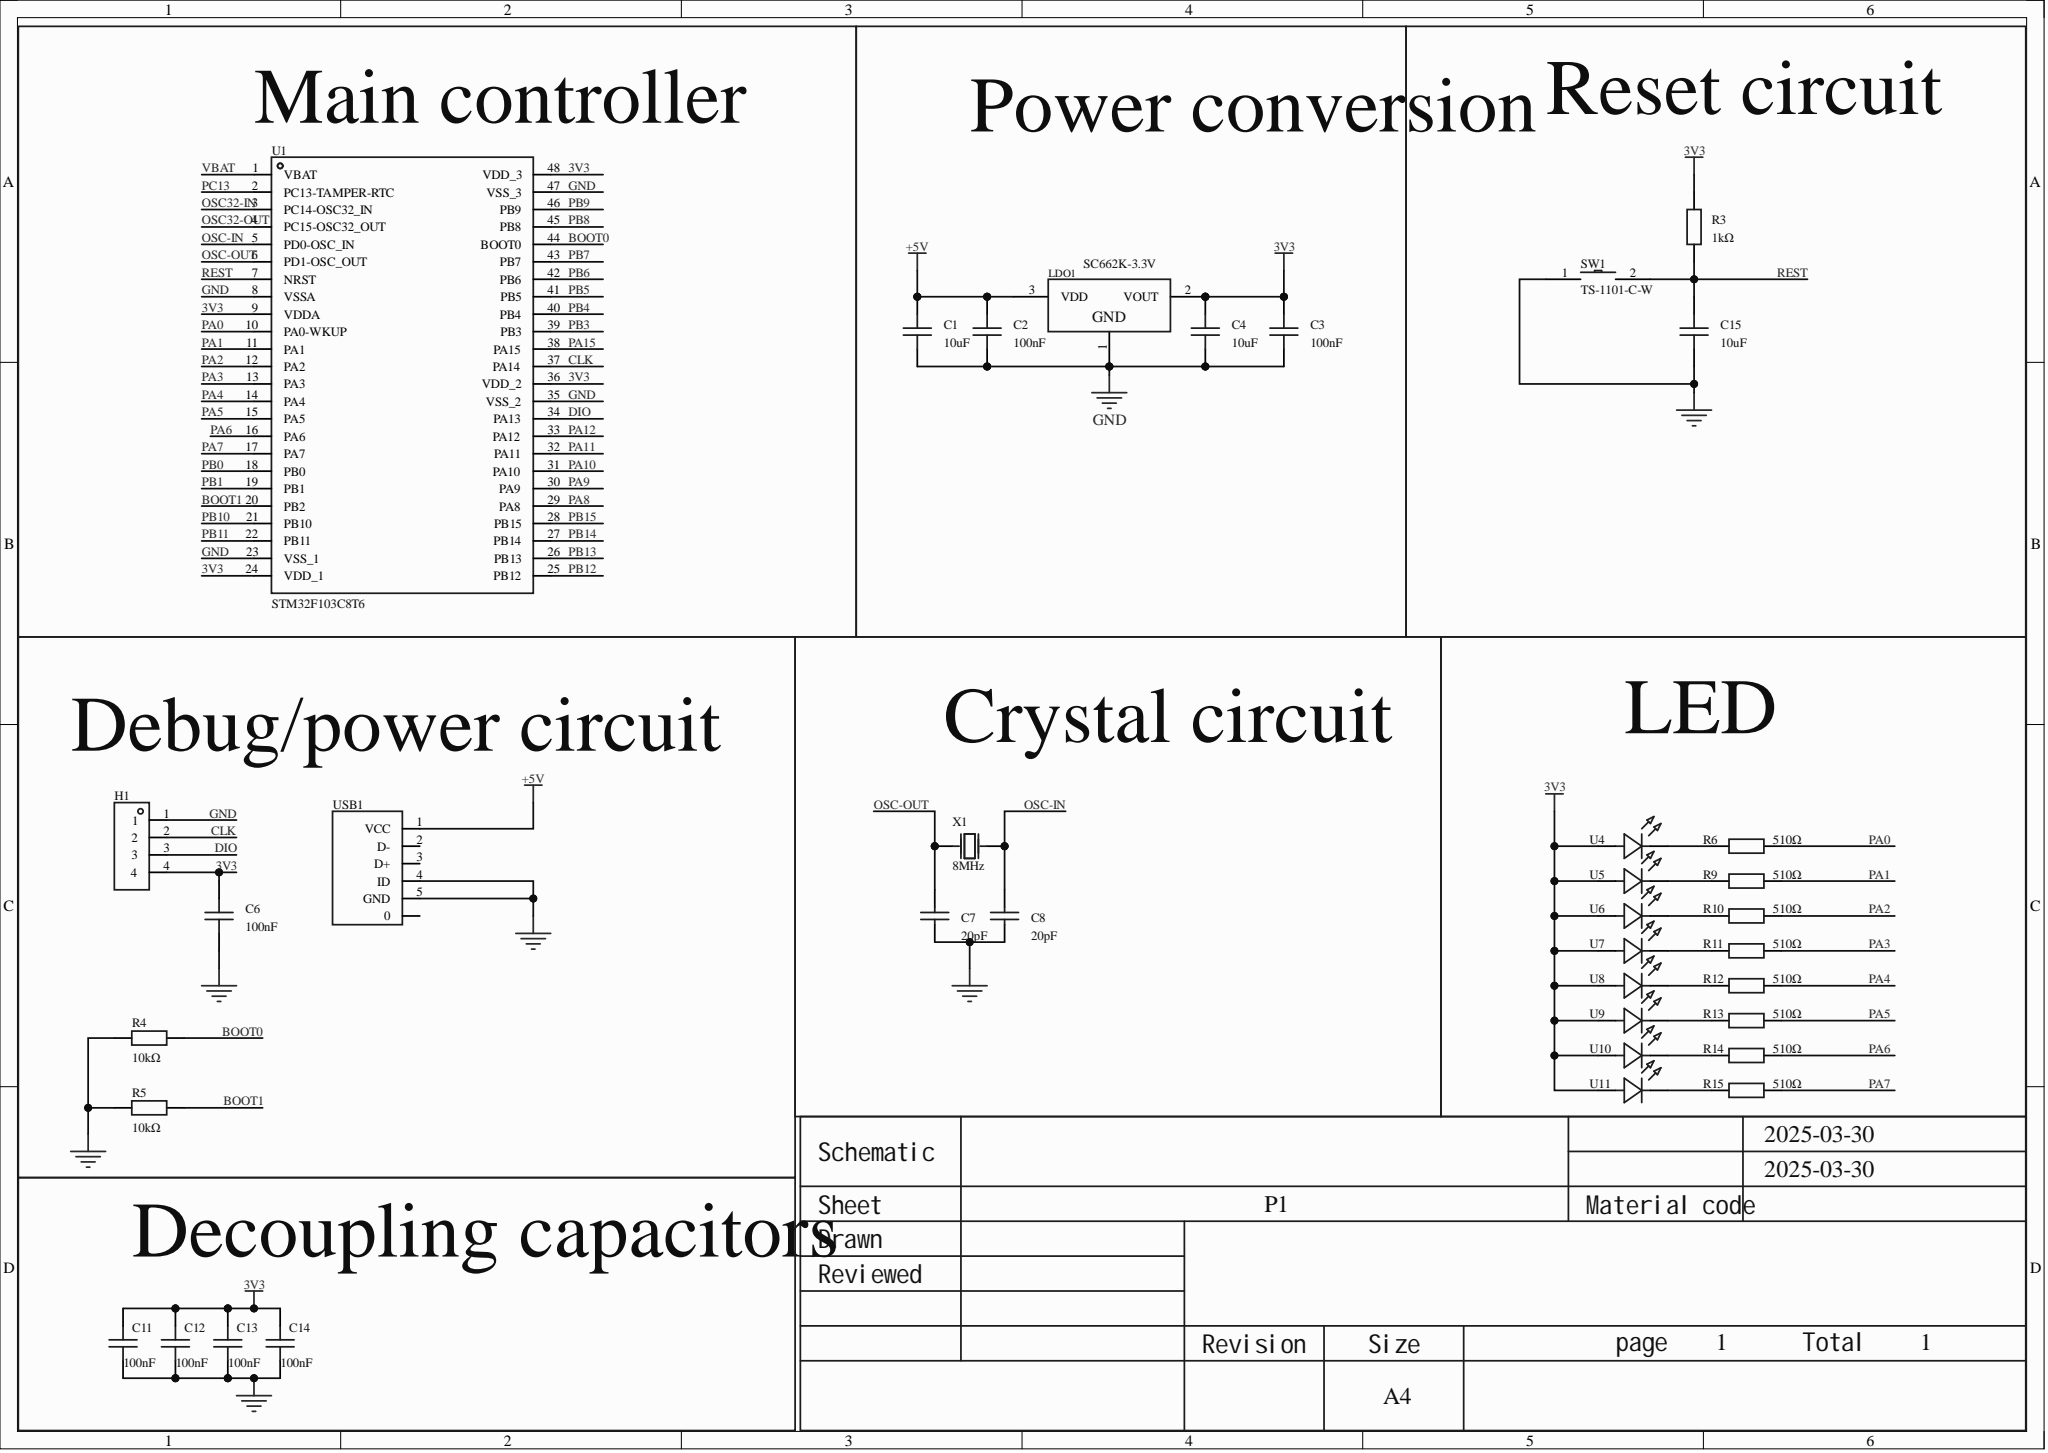Circuit board | Altium Designer | 37 parts | 26 nets
Bill of materials:
Comment,Description,Designator,Footprint,LibRef,Quantity
"10uF","Capacitance: 10uF; tolerance: ±10%; rated voltage: 10V; dielectric (temperature coefficient): X5R;","C1, C4, C15","C0603","CL10A106KP8NNNC","3"
"100nF","Capacitance: 100nF; tolerance: ±10%; rated voltage: 50V; dielectric (temperature coefficient): X7R;","C2, C3, C6, C11, C12, C13, C14","C0603","CC0603KRX7R9BB104, CGA0603X7R104K500JT","7"
"20pF","Capacitance: 20pF; tolerance: ±5%; rated voltage: 50V; dielectric (temperature coefficient): C0G;","C7, C8","C0603","CL10C200JB8NNNC","2"
"","","H1","HDR-TH_4P-P2.54-V-M","HDR-M_2.54_1x4P","1"
"SC662K-3.3V","Output type: fixed; output polarity: positive; max input voltage: 6V; output voltage: 3.3V; output current: 250mA; power supply ripple rejection (PSRR): 50dB@(1kHz);","LDO1","SOT-23-3_L2.9-W1.3-P1.90-LS2.4-BR","SC662K-3.3V","1"
"1kΩ","Resistor type: thick film resistor; resistance: 1kΩ; tolerance: ±1%; power: 100mW; max working voltage: 75V; temperature coefficient: ±100ppm/?;","R3","R0603","RC0603FR-071KL","1"
"10kΩ","Resistor type: thick film resistor; resistance: 10kΩ; tolerance: ±1%; power: 100mW; max working voltage: 75V; temperature coefficient: ±100ppm/?;","R4, R5","R0603","0603WAF1002T5E","2"
"510Ω","Resistor type: thick film resistor; resistance: 510Ω; tolerance: ±1%; power: 100mW; max working voltage: 75V; temperature coefficient: ±100ppm/?;","R6, R9, R10, R11, R12, R13, R14, R15","R0603","0603WAF5100T5E","8"
"TS-1101-C-W","Circuit structure: SPST; button shape: rectangular button; actuation force: 260gf; mounting: upright SMD; switch length: 6mm; switch width: 3.6mm; switch height: 2.5mm; with bracket: without; contact current: 50mA; rated voltage (AC): -; rated voltage (DC): 12V; rated power: -; insulation resistance: -; with lamp: none; mechanical life: 5万 cycles;","SW1","SW-SMD_L6.0-W3.3-LS8.0","TS-1101-C-W","1"
"STM32F103C8T6","CPU core: ARM-M3; program storage capacity: 64KB; RAM total: 20KB; GPIO port count: 37; operating voltage range: 2V~3.6V; max CPU frequency: 72MHz; program memory type: FLASH;","U1","LQFP-48_L7.0-W7.0-P0.50-LS9.0-BL","STM32F103C8T6","1"
"42-51/GHC-YW2X2K/3T","Emitted color: emerald green; forward current: -; dominant wavelength: 520nm~535nm; luminous intensity: 2850mcd;","U4, U5, U6, U7, U8, U9, U10, U11","LED-SMD_L1.6-W0.8-FD_GREEN-1","42-51/GHC-YW2X2K/3T","8"
"920-D62A2021S10100","Connector type: Micro-B; standard: USB 2.0; gender: female; contacts: 5P; ports: 1; rated current - power: 1A;","USB1","MICRO-USB-SMD_5P-P0.65-H-M_MICRO-USB-5P","920-D62A2021S10100","1"
"8MHz","Crystal type: through-hole crystal; frequency: 8MHz; frequency tolerance at room temperature: ±20ppm; external load capacitance: 20pF; frequency stability (full temperature): ±30ppm;","X1","OSC-TH_L10.0-W4.5-P5.00","X49SD8MSD2SC","1"
Netlist (Protel format):
[
C1
C0603
10uF



]
[
C2
C0603
100nF



]
[
C3
C0603
100nF



]
[
C4
C0603
10uF



]
[
C6
C0603
100nF



]
[
C7
C0603
20pF



]
[
C8
C0603
20pF



]
[
C11
C0603
100nF



]
[
C12
C0603
100nF



]
[
C13
C0603
100nF



]
[
C14
C0603
100nF



]
[
C15
C0603
10uF



]
[
H1
HDR-TH_4P-P2.54-V-M




]
[
LDO1
SOT-23-3_L2.9-W1.3-P1.90-LS2.4-BR
SC662K-3.3V



]
[
R3
R0603
1kΩ



]
[
R4
R0603
10kΩ



]
[
R5
R0603
10kΩ



]
[
R6
R0603
510Ω



]
[
R9
R0603
510Ω



]
[
R10
R0603
510Ω



]
[
R11
R0603
510Ω



]
[
R12
R0603
510Ω



]
[
R13
R0603
510Ω



]
[
R14
R0603
510Ω



]
[
R15
R0603
510Ω



]
[
SW1
SW-SMD_L6.0-W3.3-LS8.0
TS-1101-C-W



]
[
U1
LQFP-48_L7.0-W7.0-P0.50-LS9.0-BL
STM32F103C8T6



]
[
U4
LED-SMD_L1.6-W0.8-FD_GREEN-1
42-51/GHC-YW2X2K/3T



]
[
U5
LED-SMD_L1.6-W0.8-FD_GREEN-1
42-51/GHC-YW2X2K/3T



]
[
U6
LED-SMD_L1.6-W0.8-FD_GREEN-1
42-51/GHC-YW2X2K/3T



]
[
U7
LED-SMD_L1.6-W0.8-FD_GREEN-1
42-51/GHC-YW2X2K/3T



]
[
U8
LED-SMD_L1.6-W0.8-FD_GREEN-1
42-51/GHC-YW2X2K/3T



]
[
U9
LED-SMD_L1.6-W0.8-FD_GREEN-1
42-51/GHC-YW2X2K/3T



]
[
U10
LED-SMD_L1.6-W0.8-FD_GREEN-1
42-51/GHC-YW2X2K/3T



]
[
U11
LED-SMD_L1.6-W0.8-FD_GREEN-1
42-51/GHC-YW2X2K/3T



]
[
USB1
MICRO-USB-SMD_5P-P0.65-H-M_MICRO-USB-5P
920-D62A2021S10100



]
[
X1
OSC-TH_L10.0-W4.5-P5.00
8MHz



]
(
REST
C15-2
R3-1
SW1-2
U1-7
)
(
PA7
R15-2
U1-17
)
(
PA6
R14-2
U1-16
)
(
PA5
R13-2
U1-15
)
(
PA4
R12-2
U1-14
)
(
PA3
R11-2
U1-13
)
(
PA2
R10-2
U1-12
)
(
PA1
R9-2
U1-11
)
(
PA0
R6-2
U1-10
)
(
OSC-OUT
C7-2
U1-6
X1-2
)
(
OSC-IN
C8-2
U1-5
X1-1
)
(
NetR15_1
R15-1
U11-2
)
(
NetR14_1
R14-1
U10-2
)
(
NetR13_1
R13-1
U9-2
)
(
NetR12_1
R12-1
U8-2
)
(
NetR11_1
R11-1
U7-2
)
(
NetR10_1
R10-1
U6-2
)
(
NetR9_1
R9-1
U5-2
)
(
NetR6_1
R6-1
U4-2
)
(
GND
C1-1
C2-1
C3-1
C4-1
C6-1
C7-1
C8-1
C11-1
C12-1
C13-1
C14-1
C15-1
H1-1
LDO1-1
R4-1
R5-1
SW1-1
U1-8
U1-23
U1-35
U1-47
USB1-4
USB1-5
)
(
DIO
H1-3
U1-34
)
(
CLK
H1-2
U1-37
)
(
BOOT1
R5-2
U1-20
)
(
BOOT0
R4-2
U1-44
)
(
+5V
C1-2
C2-2
LDO1-3
USB1-1
)
(
3V3
C3-2
C4-2
C6-2
C11-2
C12-2
C13-2
C14-2
H1-4
LDO1-2
R3-2
U1-9
U1-24
U1-36
U1-48
U4-1
U5-1
U6-1
U7-1
U8-1
U9-1
U10-1
U11-1
)